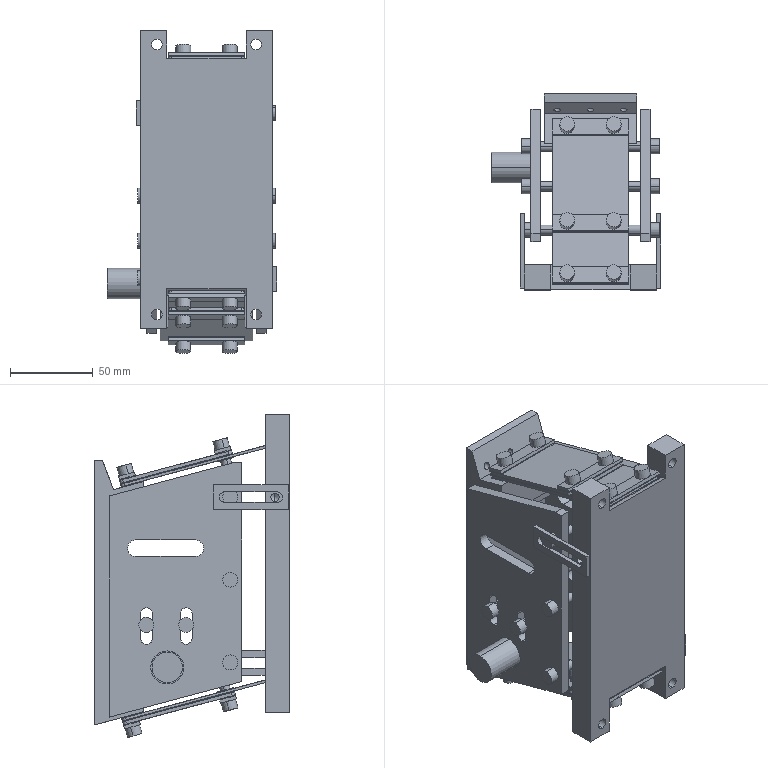Part | SolidWorks | 55 solids | 650 faces | box 102.5 x 118.189 x 195.029 mm | volume 527547 mm3 | cylinder 324 | plane 296 | cone 30 | commonest cylinder face diameters 6.5 x128 6 x44 9 x44 6.4 x26 5 x24 4 x16